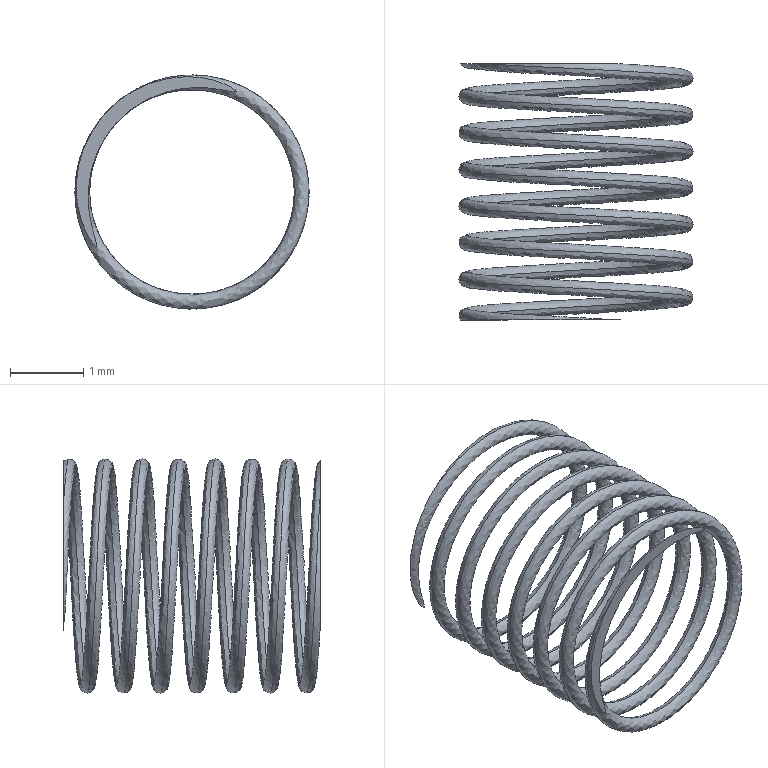Part | SolidWorks | features Helix 1, ICE 1, Sweep 1 | 1 solid | 4 faces | volume 2.155 mm3 | spline 2 | plane 2